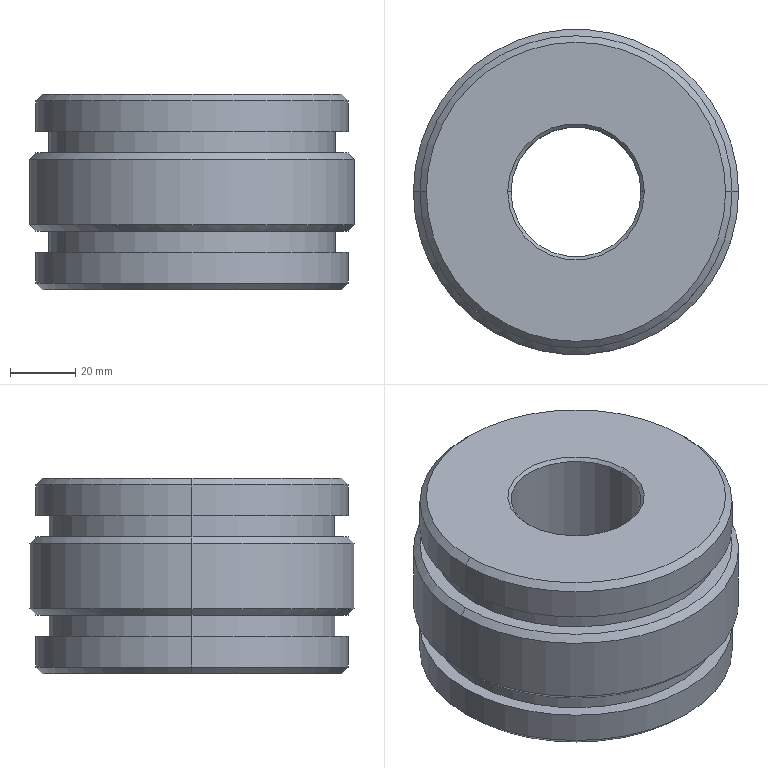Part | SolidWorks | features ICE 4, Chamfer 3, Extrusion 1 | 1 solid | 30 faces | box 100 x 100 x 60 mm | volume 356087 mm3 | cone 12 | cylinder 12 | plane 6 | commonest cylinder face diameters 88 x4 96 x4 40 x2 100 x2
STEP:
#1=CARTESIAN_POINT('',(-48.,0.,18.));
#2=VERTEX_POINT('',#1);
#3=CARTESIAN_POINT('',(48.,0.,18.));
#4=VERTEX_POINT('',#3);
#5=CARTESIAN_POINT('',(0.,0.,18.));
#6=DIRECTION('',(0.,0.,-1.));
#7=DIRECTION('',(1.,0.,0.));
#8=AXIS2_PLACEMENT_3D('',#5,#6,#7);
#9=CIRCLE('',#8,48.);
#10=EDGE_CURVE('',#2,#4,#9,.T.);
#11=ORIENTED_EDGE('',*,*,#10,.F.);
#12=CARTESIAN_POINT('',(-50.,0.,20.));
#13=VERTEX_POINT('',#12);
#14=CARTESIAN_POINT('',(-50.,0.,20.));
#15=DIRECTION('',(-0.7071,0.,0.7071));
#16=VECTOR('',#15,1000.);
#17=LINE('',#14,#16);
#18=EDGE_CURVE('',#2,#13,#17,.T.);
#19=ORIENTED_EDGE('',*,*,#18,.T.);
#20=CARTESIAN_POINT('',(50.,0.,20.));
#21=VERTEX_POINT('',#20);
#22=CARTESIAN_POINT('',(0.,0.,20.));
#23=DIRECTION('',(0.,0.,1.));
#24=DIRECTION('',(1.,0.,0.));
#25=AXIS2_PLACEMENT_3D('',#22,#23,#24);
#26=CIRCLE('',#25,50.);
#27=EDGE_CURVE('',#21,#13,#26,.T.);
#28=ORIENTED_EDGE('',*,*,#27,.F.);
#29=CARTESIAN_POINT('',(50.,0.,20.));
#30=DIRECTION('',(0.7071,0.,0.7071));
#31=VECTOR('',#30,1000.);
#32=LINE('',#29,#31);
#33=EDGE_CURVE('',#4,#21,#32,.T.);
#34=ORIENTED_EDGE('',*,*,#33,.F.);
#35=EDGE_LOOP('',(#11,#19,#28,#34));
#36=FACE_OUTER_BOUND('',#35,.T.);
#37=CARTESIAN_POINT('',(0.,0.,20.));
#38=DIRECTION('',(0.,0.,1.));
#39=DIRECTION('',(1.,0.,0.));
#40=AXIS2_PLACEMENT_3D('',#37,#38,#39);
#41=CONICAL_SURFACE('',#40,50.,0.7854);
#42=ADVANCED_FACE('',(#36),#41,.T.);
#43=CARTESIAN_POINT('',(48.,0.,42.));
#44=VERTEX_POINT('',#43);
#45=CARTESIAN_POINT('',(-48.,0.,42.));
#46=VERTEX_POINT('',#45);
#47=CARTESIAN_POINT('',(0.,0.,42.));
#48=DIRECTION('',(0.,0.,1.));
#49=DIRECTION('',(-1.,0.,0.));
#50=AXIS2_PLACEMENT_3D('',#47,#48,#49);
#51=CIRCLE('',#50,48.);
#52=EDGE_CURVE('',#44,#46,#51,.T.);
#53=ORIENTED_EDGE('',*,*,#52,.F.);
#54=CARTESIAN_POINT('',(50.,0.,40.));
#55=VERTEX_POINT('',#54);
#56=CARTESIAN_POINT('',(50.,0.,40.));
#57=DIRECTION('',(0.7071,0.,-0.7071));
#58=VECTOR('',#57,1000.);
#59=LINE('',#56,#58);
#60=EDGE_CURVE('',#44,#55,#59,.T.);
#61=ORIENTED_EDGE('',*,*,#60,.T.);
#62=CARTESIAN_POINT('',(-50.,0.,40.));
#63=VERTEX_POINT('',#62);
#64=CARTESIAN_POINT('',(0.,0.,40.));
#65=DIRECTION('',(0.,0.,-1.));
#66=DIRECTION('',(-1.,0.,0.));
#67=AXIS2_PLACEMENT_3D('',#64,#65,#66);
#68=CIRCLE('',#67,50.);
#69=EDGE_CURVE('',#63,#55,#68,.T.);
#70=ORIENTED_EDGE('',*,*,#69,.F.);
#71=CARTESIAN_POINT('',(-50.,0.,40.));
#72=DIRECTION('',(-0.7071,0.,-0.7071));
#73=VECTOR('',#72,1000.);
#74=LINE('',#71,#73);
#75=EDGE_CURVE('',#46,#63,#74,.T.);
#76=ORIENTED_EDGE('',*,*,#75,.F.);
#77=EDGE_LOOP('',(#53,#61,#70,#76));
#78=FACE_OUTER_BOUND('',#77,.T.);
#79=CARTESIAN_POINT('',(0.,0.,40.));
#80=DIRECTION('',(0.,0.,-1.));
#81=DIRECTION('',(-1.,0.,0.));
#82=AXIS2_PLACEMENT_3D('',#79,#80,#81);
#83=CONICAL_SURFACE('',#82,50.,0.7854);
#84=ADVANCED_FACE('',(#78),#83,.T.);
#85=CARTESIAN_POINT('',(20.,0.,1.));
#86=VERTEX_POINT('',#85);
#87=CARTESIAN_POINT('',(-20.,0.,1.));
#88=VERTEX_POINT('',#87);
#89=CARTESIAN_POINT('',(0.,0.,1.));
#90=DIRECTION('',(0.,0.,-1.));
#91=DIRECTION('',(1.,0.,0.));
#92=AXIS2_PLACEMENT_3D('',#89,#90,#91);
#93=CIRCLE('',#92,20.);
#94=EDGE_CURVE('',#86,#88,#93,.T.);
#95=ORIENTED_EDGE('',*,*,#94,.F.);
#96=CARTESIAN_POINT('',(21.,0.,0.));
#97=VERTEX_POINT('',#96);
#98=CARTESIAN_POINT('',(21.,0.,0.));
#99=DIRECTION('',(0.7071,0.,-0.7071));
#100=VECTOR('',#99,1000.);
#101=LINE('',#98,#100);
#102=EDGE_CURVE('',#86,#97,#101,.T.);
#103=ORIENTED_EDGE('',*,*,#102,.T.);
#104=CARTESIAN_POINT('',(-21.,0.,0.));
#105=VERTEX_POINT('',#104);
#106=CARTESIAN_POINT('',(0.,0.,0.));
#107=DIRECTION('',(0.,0.,1.));
#108=DIRECTION('',(1.,0.,0.));
#109=AXIS2_PLACEMENT_3D('',#106,#107,#108);
#110=CIRCLE('',#109,21.);
#111=EDGE_CURVE('',#105,#97,#110,.T.);
#112=ORIENTED_EDGE('',*,*,#111,.F.);
#113=CARTESIAN_POINT('',(-21.,0.,0.));
#114=DIRECTION('',(-0.7071,0.,-0.7071));
#115=VECTOR('',#114,1000.);
#116=LINE('',#113,#115);
#117=EDGE_CURVE('',#88,#105,#116,.T.);
#118=ORIENTED_EDGE('',*,*,#117,.F.);
#119=EDGE_LOOP('',(#95,#103,#112,#118));
#120=FACE_OUTER_BOUND('',#119,.T.);
#121=CARTESIAN_POINT('',(0.,0.,0.));
#122=DIRECTION('',(0.,0.,-1.));
#123=DIRECTION('',(-1.,0.,0.));
#124=AXIS2_PLACEMENT_3D('',#121,#122,#123);
#125=CONICAL_SURFACE('',#124,21.,0.7854);
#126=ADVANCED_FACE('',(#120),#125,.F.);
#127=CARTESIAN_POINT('',(-20.,0.,59.));
#128=VERTEX_POINT('',#127);
#129=CARTESIAN_POINT('',(20.,0.,59.));
#130=VERTEX_POINT('',#129);
#131=CARTESIAN_POINT('',(0.,0.,59.));
#132=DIRECTION('',(0.,0.,1.));
#133=DIRECTION('',(1.,0.,0.));
#134=AXIS2_PLACEMENT_3D('',#131,#132,#133);
#135=CIRCLE('',#134,20.);
#136=EDGE_CURVE('',#128,#130,#135,.T.);
#137=ORIENTED_EDGE('',*,*,#136,.F.);
#138=CARTESIAN_POINT('',(-21.,0.,60.));
#139=VERTEX_POINT('',#138);
#140=CARTESIAN_POINT('',(-20.,0.,59.));
#141=DIRECTION('',(-0.7071,0.,0.7071));
#142=VECTOR('',#141,1000.);
#143=LINE('',#140,#142);
#144=EDGE_CURVE('',#128,#139,#143,.T.);
#145=ORIENTED_EDGE('',*,*,#144,.T.);
#146=CARTESIAN_POINT('',(21.,0.,60.));
#147=VERTEX_POINT('',#146);
#148=CARTESIAN_POINT('',(0.,0.,60.));
#149=DIRECTION('',(0.,0.,-1.));
#150=DIRECTION('',(1.,0.,0.));
#151=AXIS2_PLACEMENT_3D('',#148,#149,#150);
#152=CIRCLE('',#151,21.);
#153=EDGE_CURVE('',#147,#139,#152,.T.);
#154=ORIENTED_EDGE('',*,*,#153,.F.);
#155=CARTESIAN_POINT('',(20.,0.,59.));
#156=DIRECTION('',(0.7071,0.,0.7071));
#157=VECTOR('',#156,1000.);
#158=LINE('',#155,#157);
#159=EDGE_CURVE('',#130,#147,#158,.T.);
#160=ORIENTED_EDGE('',*,*,#159,.F.);
#161=EDGE_LOOP('',(#137,#145,#154,#160));
#162=FACE_OUTER_BOUND('',#161,.T.);
#163=CARTESIAN_POINT('',(0.,0.,59.));
#164=DIRECTION('',(0.,0.,1.));
#165=DIRECTION('',(1.,0.,0.));
#166=AXIS2_PLACEMENT_3D('',#163,#164,#165);
#167=CONICAL_SURFACE('',#166,20.,0.7854);
#168=ADVANCED_FACE('',(#162),#167,.F.);
#169=CARTESIAN_POINT('',(-46.,0.,0.));
#170=VERTEX_POINT('',#169);
#171=CARTESIAN_POINT('',(46.,0.,0.));
#172=VERTEX_POINT('',#171);
#173=CARTESIAN_POINT('',(0.,0.,0.));
#174=DIRECTION('',(0.,0.,-1.));
#175=DIRECTION('',(1.,0.,0.));
#176=AXIS2_PLACEMENT_3D('',#173,#174,#175);
#177=CIRCLE('',#176,46.);
#178=EDGE_CURVE('',#170,#172,#177,.T.);
#179=ORIENTED_EDGE('',*,*,#178,.F.);
#180=CARTESIAN_POINT('',(-48.,0.,2.));
#181=VERTEX_POINT('',#180);
#182=CARTESIAN_POINT('',(-46.,0.,0.));
#183=DIRECTION('',(-0.7071,0.,0.7071));
#184=VECTOR('',#183,1000.);
#185=LINE('',#182,#184);
#186=EDGE_CURVE('',#170,#181,#185,.T.);
#187=ORIENTED_EDGE('',*,*,#186,.T.);
#188=CARTESIAN_POINT('',(48.,0.,2.));
#189=VERTEX_POINT('',#188);
#190=CARTESIAN_POINT('',(0.,0.,2.));
#191=DIRECTION('',(0.,0.,1.));
#192=DIRECTION('',(1.,0.,0.));
#193=AXIS2_PLACEMENT_3D('',#190,#191,#192);
#194=CIRCLE('',#193,48.);
#195=EDGE_CURVE('',#189,#181,#194,.T.);
#196=ORIENTED_EDGE('',*,*,#195,.F.);
#197=CARTESIAN_POINT('',(46.,0.,0.));
#198=DIRECTION('',(0.7071,0.,0.7071));
#199=VECTOR('',#198,1000.);
#200=LINE('',#197,#199);
#201=EDGE_CURVE('',#172,#189,#200,.T.);
#202=ORIENTED_EDGE('',*,*,#201,.F.);
#203=EDGE_LOOP('',(#179,#187,#196,#202));
#204=FACE_OUTER_BOUND('',#203,.T.);
#205=CARTESIAN_POINT('',(0.,0.,0.));
#206=DIRECTION('',(0.,0.,1.));
#207=DIRECTION('',(1.,0.,0.));
#208=AXIS2_PLACEMENT_3D('',#205,#206,#207);
#209=CONICAL_SURFACE('',#208,46.,0.7854);
#210=ADVANCED_FACE('',(#204),#209,.T.);
#211=CARTESIAN_POINT('',(46.,0.,60.));
#212=VERTEX_POINT('',#211);
#213=CARTESIAN_POINT('',(-46.,0.,60.));
#214=VERTEX_POINT('',#213);
#215=CARTESIAN_POINT('',(0.,0.,60.));
#216=DIRECTION('',(0.,0.,1.));
#217=DIRECTION('',(1.,0.,0.));
#218=AXIS2_PLACEMENT_3D('',#215,#216,#217);
#219=CIRCLE('',#218,46.);
#220=EDGE_CURVE('',#212,#214,#219,.T.);
#221=ORIENTED_EDGE('',*,*,#220,.F.);
#222=CARTESIAN_POINT('',(48.,0.,58.));
#223=VERTEX_POINT('',#222);
#224=CARTESIAN_POINT('',(46.,0.,60.));
#225=DIRECTION('',(0.7071,0.,-0.7071));
#226=VECTOR('',#225,1000.);
#227=LINE('',#224,#226);
#228=EDGE_CURVE('',#212,#223,#227,.T.);
#229=ORIENTED_EDGE('',*,*,#228,.T.);
#230=CARTESIAN_POINT('',(-48.,0.,58.));
#231=VERTEX_POINT('',#230);
#232=CARTESIAN_POINT('',(0.,0.,58.));
#233=DIRECTION('',(0.,0.,-1.));
#234=DIRECTION('',(1.,0.,0.));
#235=AXIS2_PLACEMENT_3D('',#232,#233,#234);
#236=CIRCLE('',#235,48.);
#237=EDGE_CURVE('',#231,#223,#236,.T.);
#238=ORIENTED_EDGE('',*,*,#237,.F.);
#239=CARTESIAN_POINT('',(-46.,0.,60.));
#240=DIRECTION('',(-0.7071,0.,-0.7071));
#241=VECTOR('',#240,1000.);
#242=LINE('',#239,#241);
#243=EDGE_CURVE('',#214,#231,#242,.T.);
#244=ORIENTED_EDGE('',*,*,#243,.F.);
#245=EDGE_LOOP('',(#221,#229,#238,#244));
#246=FACE_OUTER_BOUND('',#245,.T.);
#247=CARTESIAN_POINT('',(0.,0.,60.));
#248=DIRECTION('',(0.,0.,-1.));
#249=DIRECTION('',(-1.,0.,0.));
#250=AXIS2_PLACEMENT_3D('',#247,#248,#249);
#251=CONICAL_SURFACE('',#250,46.,0.7854);
#252=ADVANCED_FACE('',(#246),#251,.T.);
#253=CARTESIAN_POINT('',(48.,0.,11.5));
#254=VERTEX_POINT('',#253);
#255=CARTESIAN_POINT('',(-48.,0.,11.5));
#256=VERTEX_POINT('',#255);
#257=CARTESIAN_POINT('',(0.,0.,11.5));
#258=DIRECTION('',(0.,0.,1.));
#259=DIRECTION('',(1.,0.,0.));
#260=AXIS2_PLACEMENT_3D('',#257,#258,#259);
#261=CIRCLE('',#260,48.);
#262=EDGE_CURVE('',#254,#256,#261,.T.);
#263=ORIENTED_EDGE('',*,*,#262,.F.);
#264=CARTESIAN_POINT('',(48.,0.,12.));
#265=DIRECTION('',(0.,0.,-1.));
#266=VECTOR('',#265,1000.);
#267=LINE('',#264,#266);
#268=EDGE_CURVE('',#254,#189,#267,.T.);
#269=ORIENTED_EDGE('',*,*,#268,.T.);
#270=ORIENTED_EDGE('',*,*,#195,.T.);
#271=CARTESIAN_POINT('',(-48.,0.,12.));
#272=DIRECTION('',(0.,0.,-1.));
#273=VECTOR('',#272,1000.);
#274=LINE('',#271,#273);
#275=EDGE_CURVE('',#256,#181,#274,.T.);
#276=ORIENTED_EDGE('',*,*,#275,.F.);
#277=EDGE_LOOP('',(#263,#269,#270,#276));
#278=FACE_OUTER_BOUND('',#277,.T.);
#279=CARTESIAN_POINT('',(0.,0.,12.));
#280=DIRECTION('',(0.,0.,-1.));
#281=DIRECTION('',(-1.,0.,0.));
#282=AXIS2_PLACEMENT_3D('',#279,#280,#281);
#283=CYLINDRICAL_SURFACE('',#282,48.);
#284=ADVANCED_FACE('',(#278),#283,.T.);
#285=CARTESIAN_POINT('',(-48.,0.,48.5));
#286=VERTEX_POINT('',#285);
#287=CARTESIAN_POINT('',(48.,0.,48.5));
#288=VERTEX_POINT('',#287);
#289=CARTESIAN_POINT('',(0.,0.,48.5));
#290=DIRECTION('',(0.,0.,-1.));
#291=DIRECTION('',(-1.,0.,0.));
#292=AXIS2_PLACEMENT_3D('',#289,#290,#291);
#293=CIRCLE('',#292,48.);
#294=EDGE_CURVE('',#286,#288,#293,.T.);
#295=ORIENTED_EDGE('',*,*,#294,.F.);
#296=CARTESIAN_POINT('',(-48.,0.,48.));
#297=DIRECTION('',(0.,0.,1.));
#298=VECTOR('',#297,1000.);
#299=LINE('',#296,#298);
#300=EDGE_CURVE('',#286,#231,#299,.T.);
#301=ORIENTED_EDGE('',*,*,#300,.T.);
#302=ORIENTED_EDGE('',*,*,#237,.T.);
#303=CARTESIAN_POINT('',(48.,0.,48.));
#304=DIRECTION('',(0.,0.,1.));
#305=VECTOR('',#304,1000.);
#306=LINE('',#303,#305);
#307=EDGE_CURVE('',#288,#223,#306,.T.);
#308=ORIENTED_EDGE('',*,*,#307,.F.);
#309=EDGE_LOOP('',(#295,#301,#302,#308));
#310=FACE_OUTER_BOUND('',#309,.T.);
#311=CARTESIAN_POINT('',(0.,0.,48.));
#312=DIRECTION('',(0.,0.,1.));
#313=DIRECTION('',(1.,0.,0.));
#314=AXIS2_PLACEMENT_3D('',#311,#312,#313);
#315=CYLINDRICAL_SURFACE('',#314,48.);
#316=ADVANCED_FACE('',(#310),#315,.T.);
#317=CARTESIAN_POINT('',(44.,0.,18.));
#318=VERTEX_POINT('',#317);
#319=CARTESIAN_POINT('',(-44.,0.,18.));
#320=VERTEX_POINT('',#319);
#321=CARTESIAN_POINT('',(0.,0.,18.));
#322=DIRECTION('',(0.,0.,1.));
#323=DIRECTION('',(1.,0.,0.));
#324=AXIS2_PLACEMENT_3D('',#321,#322,#323);
#325=CIRCLE('',#324,44.);
#326=EDGE_CURVE('',#318,#320,#325,.T.);
#327=ORIENTED_EDGE('',*,*,#326,.F.);
#328=CARTESIAN_POINT('',(44.,0.,11.5));
#329=VERTEX_POINT('',#328);
#330=CARTESIAN_POINT('',(44.,0.,18.));
#331=DIRECTION('',(0.,0.,-1.));
#332=VECTOR('',#331,1000.);
#333=LINE('',#330,#332);
#334=EDGE_CURVE('',#318,#329,#333,.T.);
#335=ORIENTED_EDGE('',*,*,#334,.T.);
#336=CARTESIAN_POINT('',(-44.,0.,11.5));
#337=VERTEX_POINT('',#336);
#338=CARTESIAN_POINT('',(0.,0.,11.5));
#339=DIRECTION('',(0.,0.,1.));
#340=DIRECTION('',(1.,0.,0.));
#341=AXIS2_PLACEMENT_3D('',#338,#339,#340);
#342=CIRCLE('',#341,44.);
#343=EDGE_CURVE('',#329,#337,#342,.T.);
#344=ORIENTED_EDGE('',*,*,#343,.T.);
#345=CARTESIAN_POINT('',(-44.,0.,18.));
#346=DIRECTION('',(0.,0.,-1.));
#347=VECTOR('',#346,1000.);
#348=LINE('',#345,#347);
#349=EDGE_CURVE('',#320,#337,#348,.T.);
#350=ORIENTED_EDGE('',*,*,#349,.F.);
#351=EDGE_LOOP('',(#327,#335,#344,#350));
#352=FACE_OUTER_BOUND('',#351,.T.);
#353=CARTESIAN_POINT('',(0.,0.,18.));
#354=DIRECTION('',(0.,0.,-1.));
#355=DIRECTION('',(-1.,0.,0.));
#356=AXIS2_PLACEMENT_3D('',#353,#354,#355);
#357=CYLINDRICAL_SURFACE('',#356,44.);
#358=ADVANCED_FACE('',(#352),#357,.T.);
#359=CARTESIAN_POINT('',(-44.,0.,48.5));
#360=VERTEX_POINT('',#359);
#361=CARTESIAN_POINT('',(44.,0.,48.5));
#362=VERTEX_POINT('',#361);
#363=CARTESIAN_POINT('',(0.,0.,48.5));
#364=DIRECTION('',(0.,0.,-1.));
#365=DIRECTION('',(-1.,0.,0.));
#366=AXIS2_PLACEMENT_3D('',#363,#364,#365);
#367=CIRCLE('',#366,44.);
#368=EDGE_CURVE('',#360,#362,#367,.T.);
#369=ORIENTED_EDGE('',*,*,#368,.T.);
#370=CARTESIAN_POINT('',(44.,0.,42.));
#371=VERTEX_POINT('',#370);
#372=CARTESIAN_POINT('',(44.,0.,48.5));
#373=DIRECTION('',(0.,0.,-1.));
#374=VECTOR('',#373,1000.);
#375=LINE('',#372,#374);
#376=EDGE_CURVE('',#362,#371,#375,.T.);
#377=ORIENTED_EDGE('',*,*,#376,.T.);
#378=CARTESIAN_POINT('',(-44.,0.,42.));
#379=VERTEX_POINT('',#378);
#380=CARTESIAN_POINT('',(0.,0.,42.));
#381=DIRECTION('',(0.,0.,-1.));
#382=DIRECTION('',(-1.,0.,0.));
#383=AXIS2_PLACEMENT_3D('',#380,#381,#382);
#384=CIRCLE('',#383,44.);
#385=EDGE_CURVE('',#379,#371,#384,.T.);
#386=ORIENTED_EDGE('',*,*,#385,.F.);
#387=CARTESIAN_POINT('',(-44.,0.,48.5));
#388=DIRECTION('',(0.,0.,-1.));
#389=VECTOR('',#388,1000.);
#390=LINE('',#387,#389);
#391=EDGE_CURVE('',#360,#379,#390,.T.);
#392=ORIENTED_EDGE('',*,*,#391,.F.);
#393=EDGE_LOOP('',(#369,#377,#386,#392));
#394=FACE_OUTER_BOUND('',#393,.T.);
#395=CARTESIAN_POINT('',(0.,0.,48.5));
#396=DIRECTION('',(0.,0.,-1.));
#397=DIRECTION('',(-1.,0.,0.));
#398=AXIS2_PLACEMENT_3D('',#395,#396,#397);
#399=CYLINDRICAL_SURFACE('',#398,44.);
#400=ADVANCED_FACE('',(#394),#399,.T.);
#401=ORIENTED_EDGE('',*,*,#136,.T.);
#402=CARTESIAN_POINT('',(20.,0.,60.));
#403=DIRECTION('',(0.,0.,-1.));
#404=VECTOR('',#403,1000.);
#405=LINE('',#402,#404);
#406=EDGE_CURVE('',#130,#86,#405,.T.);
#407=ORIENTED_EDGE('',*,*,#406,.T.);
#408=ORIENTED_EDGE('',*,*,#94,.T.);
#409=CARTESIAN_POINT('',(-20.,0.,60.));
#410=DIRECTION('',(0.,0.,-1.));
#411=VECTOR('',#410,1000.);
#412=LINE('',#409,#411);
#413=EDGE_CURVE('',#128,#88,#412,.T.);
#414=ORIENTED_EDGE('',*,*,#413,.F.);
#415=EDGE_LOOP('',(#401,#407,#408,#414));
#416=FACE_OUTER_BOUND('',#415,.T.);
#417=CARTESIAN_POINT('',(0.,0.,60.));
#418=DIRECTION('',(0.,0.,-1.));
#419=DIRECTION('',(-1.,0.,0.));
#420=AXIS2_PLACEMENT_3D('',#417,#418,#419);
#421=CYLINDRICAL_SURFACE('',#420,20.);
#422=ADVANCED_FACE('',(#416),#421,.F.);
#423=ORIENTED_EDGE('',*,*,#69,.T.);
#424=CARTESIAN_POINT('',(50.,0.,60.));
#425=DIRECTION('',(0.,0.,-1.));
#426=VECTOR('',#425,1000.);
#427=LINE('',#424,#426);
#428=EDGE_CURVE('',#55,#21,#427,.T.);
#429=ORIENTED_EDGE('',*,*,#428,.T.);
#430=ORIENTED_EDGE('',*,*,#27,.T.);
#431=CARTESIAN_POINT('',(-50.,0.,60.));
#432=DIRECTION('',(0.,0.,-1.));
#433=VECTOR('',#432,1000.);
#434=LINE('',#431,#433);
#435=EDGE_CURVE('',#63,#13,#434,.T.);
#436=ORIENTED_EDGE('',*,*,#435,.F.);
#437=EDGE_LOOP('',(#423,#429,#430,#436));
#438=FACE_OUTER_BOUND('',#437,.T.);
#439=CARTESIAN_POINT('',(0.,0.,60.));
#440=DIRECTION('',(0.,0.,-1.));
#441=DIRECTION('',(-1.,0.,0.));
#442=AXIS2_PLACEMENT_3D('',#439,#440,#441);
#443=CYLINDRICAL_SURFACE('',#442,50.);
#444=ADVANCED_FACE('',(#438),#443,.T.);
#445=ORIENTED_EDGE('',*,*,#111,.T.);
#446=CARTESIAN_POINT('',(0.,0.,0.));
#447=DIRECTION('',(0.,0.,1.));
#448=DIRECTION('',(1.,0.,0.));
#449=AXIS2_PLACEMENT_3D('',#446,#447,#448);
#450=CIRCLE('',#449,21.);
#451=EDGE_CURVE('',#97,#105,#450,.T.);
#452=ORIENTED_EDGE('',*,*,#451,.T.);
#453=EDGE_LOOP('',(#445,#452));
#454=FACE_BOUND('',#453,.T.);
#455=CARTESIAN_POINT('',(0.,0.,0.));
#456=DIRECTION('',(0.,0.,-1.));
#457=DIRECTION('',(1.,0.,0.));
#458=AXIS2_PLACEMENT_3D('',#455,#456,#457);
#459=CIRCLE('',#458,46.);
#460=EDGE_CURVE('',#172,#170,#459,.T.);
#461=ORIENTED_EDGE('',*,*,#460,.T.);
#462=ORIENTED_EDGE('',*,*,#178,.T.);
#463=EDGE_LOOP('',(#461,#462));
#464=FACE_OUTER_BOUND('',#463,.T.);
#465=CARTESIAN_POINT('',(0.,0.,0.));
#466=DIRECTION('',(0.,0.,1.));
#467=DIRECTION('',(1.,0.,0.));
#468=AXIS2_PLACEMENT_3D('',#465,#466,#467);
#469=PLANE('',#468);
#470=ADVANCED_FACE('',(#454,#464),#469,.F.);
#471=CARTESIAN_POINT('',(0.,0.,11.5));
#472=DIRECTION('',(0.,0.,1.));
#473=DIRECTION('',(1.,0.,0.));
#474=AXIS2_PLACEMENT_3D('',#471,#472,#473);
#475=CIRCLE('',#474,44.);
#476=EDGE_CURVE('',#337,#329,#475,.T.);
#477=ORIENTED_EDGE('',*,*,#476,.F.);
#478=ORIENTED_EDGE('',*,*,#343,.F.);
#479=EDGE_LOOP('',(#477,#478));
#480=FACE_BOUND('',#479,.T.);
#481=CARTESIAN_POINT('',(0.,0.,11.5));
#482=DIRECTION('',(0.,0.,1.));
#483=DIRECTION('',(1.,0.,0.));
#484=AXIS2_PLACEMENT_3D('',#481,#482,#483);
#485=CIRCLE('',#484,48.);
#486=EDGE_CURVE('',#256,#254,#485,.T.);
#487=ORIENTED_EDGE('',*,*,#486,.T.);
#488=ORIENTED_EDGE('',*,*,#262,.T.);
#489=EDGE_LOOP('',(#487,#488));
#490=FACE_OUTER_BOUND('',#489,.T.);
#491=CARTESIAN_POINT('',(0.,0.,11.5));
#492=DIRECTION('',(0.,0.,1.));
#493=DIRECTION('',(1.,0.,0.));
#494=AXIS2_PLACEMENT_3D('',#491,#492,#493);
#495=PLANE('',#494);
#496=ADVANCED_FACE('',(#480,#490),#495,.T.);
#497=ORIENTED_EDGE('',*,*,#153,.T.);
#498=CARTESIAN_POINT('',(0.,0.,60.));
#499=DIRECTION('',(0.,0.,-1.));
#500=DIRECTION('',(1.,0.,0.));
#501=AXIS2_PLACEMENT_3D('',#498,#499,#500);
#502=CIRCLE('',#501,21.);
#503=EDGE_CURVE('',#139,#147,#502,.T.);
#504=ORIENTED_EDGE('',*,*,#503,.T.);
#505=EDGE_LOOP('',(#497,#504));
#506=FACE_BOUND('',#505,.T.);
#507=CARTESIAN_POINT('',(0.,0.,60.));
#508=DIRECTION('',(0.,0.,1.));
#509=DIRECTION('',(1.,0.,0.));
#510=AXIS2_PLACEMENT_3D('',#507,#508,#509);
#511=CIRCLE('',#510,46.);
#512=EDGE_CURVE('',#214,#212,#511,.T.);
#513=ORIENTED_EDGE('',*,*,#512,.T.);
#514=ORIENTED_EDGE('',*,*,#220,.T.);
#515=EDGE_LOOP('',(#513,#514));
#516=FACE_OUTER_BOUND('',#515,.T.);
#517=CARTESIAN_POINT('',(0.,0.,60.));
#518=DIRECTION('',(0.,0.,1.));
#519=DIRECTION('',(1.,0.,0.));
#520=AXIS2_PLACEMENT_3D('',#517,#518,#519);
#521=PLANE('',#520);
#522=ADVANCED_FACE('',(#506,#516),#521,.T.);
#523=ORIENTED_EDGE('',*,*,#368,.F.);
#524=CARTESIAN_POINT('',(0.,0.,48.5));
#525=DIRECTION('',(0.,0.,-1.));
#526=DIRECTION('',(-1.,0.,0.));
#527=AXIS2_PLACEMENT_3D('',#524,#525,#526);
#528=CIRCLE('',#527,44.);
#529=EDGE_CURVE('',#362,#360,#528,.T.);
#530=ORIENTED_EDGE('',*,*,#529,.F.);
#531=EDGE_LOOP('',(#523,#530));
#532=FACE_BOUND('',#531,.T.);
#533=CARTESIAN_POINT('',(0.,0.,48.5));
#534=DIRECTION('',(0.,0.,-1.));
#535=DIRECTION('',(-1.,0.,0.));
#536=AXIS2_PLACEMENT_3D('',#533,#534,#535);
#537=CIRCLE('',#536,48.);
#538=EDGE_CURVE('',#288,#286,#537,.T.);
#539=ORIENTED_EDGE('',*,*,#538,.T.);
#540=ORIENTED_EDGE('',*,*,#294,.T.);
#541=EDGE_LOOP('',(#539,#540));
#542=FACE_OUTER_BOUND('',#541,.T.);
#543=CARTESIAN_POINT('',(0.,0.,48.5));
#544=DIRECTION('',(0.,0.,-1.));
#545=DIRECTION('',(-1.,0.,0.));
#546=AXIS2_PLACEMENT_3D('',#543,#544,#545);
#547=PLANE('',#546);
#548=ADVANCED_FACE('',(#532,#542),#547,.T.);
#549=ORIENTED_EDGE('',*,*,#428,.F.);
#550=CARTESIAN_POINT('',(0.,0.,40.));
#551=DIRECTION('',(0.,0.,-1.));
#552=DIRECTION('',(-1.,0.,0.));
#553=AXIS2_PLACEMENT_3D('',#550,#551,#552);
#554=CIRCLE('',#553,50.);
#555=EDGE_CURVE('',#55,#63,#554,.T.);
#556=ORIENTED_EDGE('',*,*,#555,.T.);
#557=ORIENTED_EDGE('',*,*,#435,.T.);
#558=CARTESIAN_POINT('',(0.,0.,20.));
#559=DIRECTION('',(0.,0.,1.));
#560=DIRECTION('',(1.,0.,0.));
#561=AXIS2_PLACEMENT_3D('',#558,#559,#560);
#562=CIRCLE('',#561,50.);
#563=EDGE_CURVE('',#13,#21,#562,.T.);
#564=ORIENTED_EDGE('',*,*,#563,.T.);
#565=EDGE_LOOP('',(#549,#556,#557,#564));
#566=FACE_OUTER_BOUND('',#565,.T.);
#567=CARTESIAN_POINT('',(0.,0.,60.));
#568=DIRECTION('',(0.,0.,-1.));
#569=DIRECTION('',(-1.,0.,0.));
#570=AXIS2_PLACEMENT_3D('',#567,#568,#569);
#571=CYLINDRICAL_SURFACE('',#570,50.);
#572=ADVANCED_FACE('',(#566),#571,.T.);
#573=ORIENTED_EDGE('',*,*,#406,.F.);
#574=CARTESIAN_POINT('',(0.,0.,59.));
#575=DIRECTION('',(0.,0.,1.));
#576=DIRECTION('',(1.,0.,0.));
#577=AXIS2_PLACEMENT_3D('',#574,#575,#576);
#578=CIRCLE('',#577,20.);
#579=EDGE_CURVE('',#130,#128,#578,.T.);
#580=ORIENTED_EDGE('',*,*,#579,.T.);
#581=ORIENTED_EDGE('',*,*,#413,.T.);
#582=CARTESIAN_POINT('',(0.,0.,1.));
#583=DIRECTION('',(0.,0.,-1.));
#584=DIRECTION('',(1.,0.,0.));
#585=AXIS2_PLACEMENT_3D('',#582,#583,#584);
#586=CIRCLE('',#585,20.);
#587=EDGE_CURVE('',#88,#86,#586,.T.);
#588=ORIENTED_EDGE('',*,*,#587,.T.);
#589=EDGE_LOOP('',(#573,#580,#581,#588));
#590=FACE_OUTER_BOUND('',#589,.T.);
#591=CARTESIAN_POINT('',(0.,0.,60.));
#592=DIRECTION('',(0.,0.,-1.));
#593=DIRECTION('',(-1.,0.,0.));
#594=AXIS2_PLACEMENT_3D('',#591,#592,#593);
#595=CYLINDRICAL_SURFACE('',#594,20.);
#596=ADVANCED_FACE('',(#590),#595,.F.);
#597=CARTESIAN_POINT('',(0.,0.,42.));
#598=DIRECTION('',(0.,0.,1.));
#599=DIRECTION('',(-1.,0.,0.));
#600=AXIS2_PLACEMENT_3D('',#597,#598,#599);
#601=CIRCLE('',#600,48.);
#602=EDGE_CURVE('',#46,#44,#601,.T.);
#603=ORIENTED_EDGE('',*,*,#602,.T.);
#604=ORIENTED_EDGE('',*,*,#52,.T.);
#605=EDGE_LOOP('',(#603,#604));
#606=FACE_OUTER_BOUND('',#605,.T.);
#607=ORIENTED_EDGE('',*,*,#385,.T.);
#608=CARTESIAN_POINT('',(0.,0.,42.));
#609=DIRECTION('',(0.,0.,-1.));
#610=DIRECTION('',(-1.,0.,0.));
#611=AXIS2_PLACEMENT_3D('',#608,#609,#610);
#612=CIRCLE('',#611,44.);
#613=EDGE_CURVE('',#371,#379,#612,.T.);
#614=ORIENTED_EDGE('',*,*,#613,.T.);
#615=EDGE_LOOP('',(#607,#614));
#616=FACE_BOUND('',#615,.T.);
#617=CARTESIAN_POINT('',(0.,0.,42.));
#618=DIRECTION('',(0.,0.,-1.));
#619=DIRECTION('',(-1.,0.,0.));
#620=AXIS2_PLACEMENT_3D('',#617,#618,#619);
#621=PLANE('',#620);
#622=ADVANCED_FACE('',(#606,#616),#621,.F.);
#623=ORIENTED_EDGE('',*,*,#376,.F.);
#624=ORIENTED_EDGE('',*,*,#529,.T.);
#625=ORIENTED_EDGE('',*,*,#391,.T.);
#626=ORIENTED_EDGE('',*,*,#613,.F.);
#627=EDGE_LOOP('',(#623,#624,#625,#626));
#628=FACE_OUTER_BOUND('',#627,.T.);
#629=CARTESIAN_POINT('',(0.,0.,48.5));
#630=DIRECTION('',(0.,0.,-1.));
#631=DIRECTION('',(-1.,0.,0.));
#632=AXIS2_PLACEMENT_3D('',#629,#630,#631);
#633=CYLINDRICAL_SURFACE('',#632,44.);
#634=ADVANCED_FACE('',(#628),#633,.T.);
#635=CARTESIAN_POINT('',(0.,0.,18.));
#636=DIRECTION('',(0.,0.,-1.));
#637=DIRECTION('',(1.,0.,0.));
#638=AXIS2_PLACEMENT_3D('',#635,#636,#637);
#639=CIRCLE('',#638,48.);
#640=EDGE_CURVE('',#4,#2,#639,.T.);
#641=ORIENTED_EDGE('',*,*,#640,.T.);
#642=ORIENTED_EDGE('',*,*,#10,.T.);
#643=EDGE_LOOP('',(#641,#642));
#644=FACE_OUTER_BOUND('',#643,.T.);
#645=CARTESIAN_POINT('',(0.,0.,18.));
#646=DIRECTION('',(0.,0.,1.));
#647=DIRECTION('',(1.,0.,0.));
#648=AXIS2_PLACEMENT_3D('',#645,#646,#647);
#649=CIRCLE('',#648,44.);
#650=EDGE_CURVE('',#320,#318,#649,.T.);
#651=ORIENTED_EDGE('',*,*,#650,.T.);
#652=ORIENTED_EDGE('',*,*,#326,.T.);
#653=EDGE_LOOP('',(#651,#652));
#654=FACE_BOUND('',#653,.T.);
#655=CARTESIAN_POINT('',(0.,0.,18.));
#656=DIRECTION('',(0.,0.,1.));
#657=DIRECTION('',(1.,0.,0.));
#658=AXIS2_PLACEMENT_3D('',#655,#656,#657);
#659=PLANE('',#658);
#660=ADVANCED_FACE('',(#644,#654),#659,.F.);
#661=ORIENTED_EDGE('',*,*,#334,.F.);
#662=ORIENTED_EDGE('',*,*,#650,.F.);
#663=ORIENTED_EDGE('',*,*,#349,.T.);
#664=ORIENTED_EDGE('',*,*,#476,.T.);
#665=EDGE_LOOP('',(#661,#662,#663,#664));
#666=FACE_OUTER_BOUND('',#665,.T.);
#667=CARTESIAN_POINT('',(0.,0.,18.));
#668=DIRECTION('',(0.,0.,-1.));
#669=DIRECTION('',(-1.,0.,0.));
#670=AXIS2_PLACEMENT_3D('',#667,#668,#669);
#671=CYLINDRICAL_SURFACE('',#670,44.);
#672=ADVANCED_FACE('',(#666),#671,.T.);
#673=ORIENTED_EDGE('',*,*,#300,.F.);
#674=ORIENTED_EDGE('',*,*,#538,.F.);
#675=ORIENTED_EDGE('',*,*,#307,.T.);
#676=CARTESIAN_POINT('',(0.,0.,58.));
#677=DIRECTION('',(0.,0.,-1.));
#678=DIRECTION('',(1.,0.,0.));
#679=AXIS2_PLACEMENT_3D('',#676,#677,#678);
#680=CIRCLE('',#679,48.);
#681=EDGE_CURVE('',#223,#231,#680,.T.);
#682=ORIENTED_EDGE('',*,*,#681,.T.);
#683=EDGE_LOOP('',(#673,#674,#675,#682));
#684=FACE_OUTER_BOUND('',#683,.T.);
#685=CARTESIAN_POINT('',(0.,0.,48.));
#686=DIRECTION('',(0.,0.,1.));
#687=DIRECTION('',(1.,0.,0.));
#688=AXIS2_PLACEMENT_3D('',#685,#686,#687);
#689=CYLINDRICAL_SURFACE('',#688,48.);
#690=ADVANCED_FACE('',(#684),#689,.T.);
#691=ORIENTED_EDGE('',*,*,#268,.F.);
#692=ORIENTED_EDGE('',*,*,#486,.F.);
#693=ORIENTED_EDGE('',*,*,#275,.T.);
#694=CARTESIAN_POINT('',(0.,0.,2.));
#695=DIRECTION('',(0.,0.,1.));
#696=DIRECTION('',(1.,0.,0.));
#697=AXIS2_PLACEMENT_3D('',#694,#695,#696);
#698=CIRCLE('',#697,48.);
#699=EDGE_CURVE('',#181,#189,#698,.T.);
#700=ORIENTED_EDGE('',*,*,#699,.T.);
#701=EDGE_LOOP('',(#691,#692,#693,#700));
#702=FACE_OUTER_BOUND('',#701,.T.);
#703=CARTESIAN_POINT('',(0.,0.,12.));
#704=DIRECTION('',(0.,0.,-1.));
#705=DIRECTION('',(-1.,0.,0.));
#706=AXIS2_PLACEMENT_3D('',#703,#704,#705);
#707=CYLINDRICAL_SURFACE('',#706,48.);
#708=ADVANCED_FACE('',(#702),#707,.T.);
#709=ORIENTED_EDGE('',*,*,#228,.F.);
#710=ORIENTED_EDGE('',*,*,#512,.F.);
#711=ORIENTED_EDGE('',*,*,#243,.T.);
#712=ORIENTED_EDGE('',*,*,#681,.F.);
#713=EDGE_LOOP('',(#709,#710,#711,#712));
#714=FACE_OUTER_BOUND('',#713,.T.);
#715=CARTESIAN_POINT('',(0.,0.,60.));
#716=DIRECTION('',(0.,0.,-1.));
#717=DIRECTION('',(-1.,0.,0.));
#718=AXIS2_PLACEMENT_3D('',#715,#716,#717);
#719=CONICAL_SURFACE('',#718,46.,0.7854);
#720=ADVANCED_FACE('',(#714),#719,.T.);
#721=ORIENTED_EDGE('',*,*,#186,.F.);
#722=ORIENTED_EDGE('',*,*,#460,.F.);
#723=ORIENTED_EDGE('',*,*,#201,.T.);
#724=ORIENTED_EDGE('',*,*,#699,.F.);
#725=EDGE_LOOP('',(#721,#722,#723,#724));
#726=FACE_OUTER_BOUND('',#725,.T.);
#727=CARTESIAN_POINT('',(0.,0.,0.));
#728=DIRECTION('',(0.,0.,1.));
#729=DIRECTION('',(1.,0.,0.));
#730=AXIS2_PLACEMENT_3D('',#727,#728,#729);
#731=CONICAL_SURFACE('',#730,46.,0.7854);
#732=ADVANCED_FACE('',(#726),#731,.T.);
#733=ORIENTED_EDGE('',*,*,#144,.F.);
#734=ORIENTED_EDGE('',*,*,#579,.F.);
#735=ORIENTED_EDGE('',*,*,#159,.T.);
#736=ORIENTED_EDGE('',*,*,#503,.F.);
#737=EDGE_LOOP('',(#733,#734,#735,#736));
#738=FACE_OUTER_BOUND('',#737,.T.);
#739=CARTESIAN_POINT('',(0.,0.,59.));
#740=DIRECTION('',(0.,0.,1.));
#741=DIRECTION('',(1.,0.,0.));
#742=AXIS2_PLACEMENT_3D('',#739,#740,#741);
#743=CONICAL_SURFACE('',#742,20.,0.7854);
#744=ADVANCED_FACE('',(#738),#743,.F.);
#745=ORIENTED_EDGE('',*,*,#102,.F.);
#746=ORIENTED_EDGE('',*,*,#587,.F.);
#747=ORIENTED_EDGE('',*,*,#117,.T.);
#748=ORIENTED_EDGE('',*,*,#451,.F.);
#749=EDGE_LOOP('',(#745,#746,#747,#748));
#750=FACE_OUTER_BOUND('',#749,.T.);
#751=CARTESIAN_POINT('',(0.,0.,0.));
#752=DIRECTION('',(0.,0.,-1.));
#753=DIRECTION('',(-1.,0.,0.));
#754=AXIS2_PLACEMENT_3D('',#751,#752,#753);
#755=CONICAL_SURFACE('',#754,21.,0.7854);
#756=ADVANCED_FACE('',(#750),#755,.F.);
#757=ORIENTED_EDGE('',*,*,#60,.F.);
#758=ORIENTED_EDGE('',*,*,#602,.F.);
#759=ORIENTED_EDGE('',*,*,#75,.T.);
#760=ORIENTED_EDGE('',*,*,#555,.F.);
#761=EDGE_LOOP('',(#757,#758,#759,#760));
#762=FACE_OUTER_BOUND('',#761,.T.);
#763=CARTESIAN_POINT('',(0.,0.,40.));
#764=DIRECTION('',(0.,0.,-1.));
#765=DIRECTION('',(-1.,0.,0.));
#766=AXIS2_PLACEMENT_3D('',#763,#764,#765);
#767=CONICAL_SURFACE('',#766,50.,0.7854);
#768=ADVANCED_FACE('',(#762),#767,.T.);
#769=ORIENTED_EDGE('',*,*,#18,.F.);
#770=ORIENTED_EDGE('',*,*,#640,.F.);
#771=ORIENTED_EDGE('',*,*,#33,.T.);
#772=ORIENTED_EDGE('',*,*,#563,.F.);
#773=EDGE_LOOP('',(#769,#770,#771,#772));
#774=FACE_OUTER_BOUND('',#773,.T.);
#775=CARTESIAN_POINT('',(0.,0.,20.));
#776=DIRECTION('',(0.,0.,1.));
#777=DIRECTION('',(1.,0.,0.));
#778=AXIS2_PLACEMENT_3D('',#775,#776,#777);
#779=CONICAL_SURFACE('',#778,50.,0.7854);
#780=ADVANCED_FACE('',(#774),#779,.T.);
#781=CLOSED_SHELL('',(#42,#84,#126,#168,#210,#252,#284,#316,#358,#400,#422,#444,#470,#496,#522,#548,#572,#596,#622,#634,#660,#672,#690,#708,#720,#732,#744,#756,#768,#780));
#782=MANIFOLD_SOLID_BREP('',#781);
#783=CARTESIAN_POINT('',(0.,0.,0.));
#784=DIRECTION('',(0.,0.,1.));
#785=DIRECTION('',(1.,0.,0.));
#786=AXIS2_PLACEMENT_3D('',#783,#784,#785);
#787=(LENGTH_UNIT()NAMED_UNIT(*)SI_UNIT(.MILLI.,.METRE.));
#788=UNCERTAINTY_MEASURE_WITH_UNIT(LENGTH_MEASURE(0.00001),#787,'','');
#789=(NAMED_UNIT(*)PLANE_ANGLE_UNIT()SI_UNIT($,.RADIAN.));
#790=(NAMED_UNIT(*)SI_UNIT($,.STERADIAN.)SOLID_ANGLE_UNIT());
#791=(GEOMETRIC_REPRESENTATION_CONTEXT(3)GLOBAL_UNCERTAINTY_ASSIGNED_CONTEXT((#788))GLOBAL_UNIT_ASSIGNED_CONTEXT((#787,#789,#790))REPRESENTATION_CONTEXT('',''));
#792=ADVANCED_BREP_SHAPE_REPRESENTATION('',(#782,#786),#791);